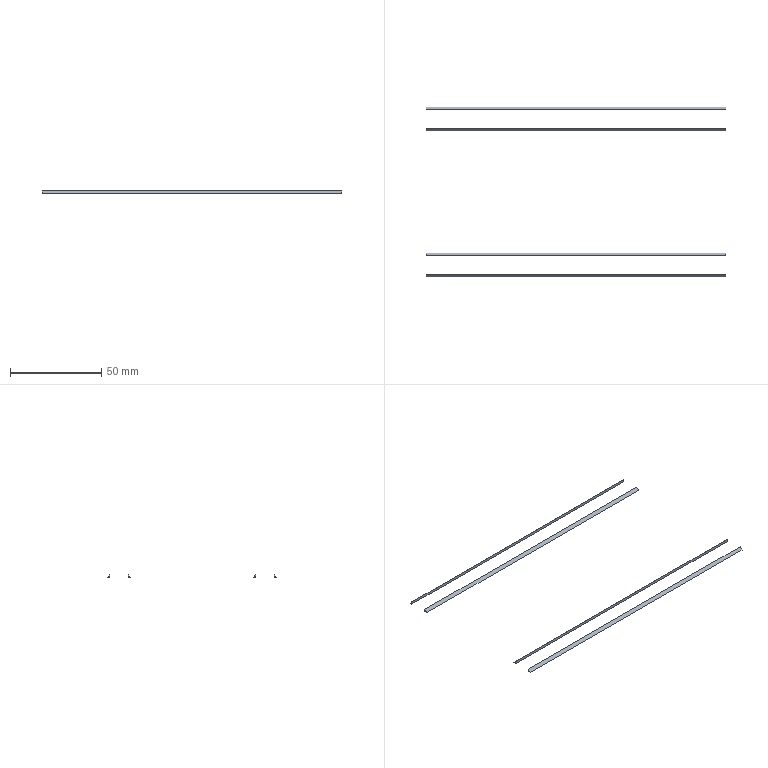Part | SolidWorks | features BaseBody 4 | 4 solids | 20 faces | box 164 x 93 x 1.5 mm | volume 738 mm3 | plane 20
STEP:
#1=CARTESIAN_POINT('',(152.,3.,6.4));
#2=VERTEX_POINT('',#1);
#3=CARTESIAN_POINT('',(152.,4.5,7.9));
#4=VERTEX_POINT('',#3);
#5=CARTESIAN_POINT('',(152.,4.5,7.9));
#6=DIRECTION('',(0.,0.7071,0.7071));
#7=VECTOR('',#6,1000.);
#8=LINE('',#5,#7);
#9=EDGE_CURVE('',#2,#4,#8,.T.);
#10=ORIENTED_EDGE('',*,*,#9,.T.);
#11=CARTESIAN_POINT('',(-12.,4.5,7.9));
#12=VERTEX_POINT('',#11);
#13=CARTESIAN_POINT('',(152.,4.5,7.9));
#14=DIRECTION('',(-1.,0.,0.));
#15=VECTOR('',#14,1000.);
#16=LINE('',#13,#15);
#17=EDGE_CURVE('',#4,#12,#16,.T.);
#18=ORIENTED_EDGE('',*,*,#17,.T.);
#19=CARTESIAN_POINT('',(-12.,3.,6.4));
#20=VERTEX_POINT('',#19);
#21=CARTESIAN_POINT('',(-12.,4.5,7.9));
#22=DIRECTION('',(0.,-0.7071,-0.7071));
#23=VECTOR('',#22,1000.);
#24=LINE('',#21,#23);
#25=EDGE_CURVE('',#12,#20,#24,.T.);
#26=ORIENTED_EDGE('',*,*,#25,.T.);
#27=CARTESIAN_POINT('',(152.,3.,6.4));
#28=DIRECTION('',(1.,0.,0.));
#29=VECTOR('',#28,1000.);
#30=LINE('',#27,#29);
#31=EDGE_CURVE('',#20,#2,#30,.T.);
#32=ORIENTED_EDGE('',*,*,#31,.T.);
#33=EDGE_LOOP('',(#10,#18,#26,#32));
#34=FACE_OUTER_BOUND('',#33,.T.);
#35=CARTESIAN_POINT('',(152.,4.5,7.9));
#36=DIRECTION('',(0.,-0.7071,0.7071));
#37=DIRECTION('',(0.,-0.7071,-0.7071));
#38=AXIS2_PLACEMENT_3D('',#35,#36,#37);
#39=PLANE('',#38);
#40=ADVANCED_FACE('',(#34),#39,.T.);
#41=CARTESIAN_POINT('',(152.,4.5,6.4));
#42=VERTEX_POINT('',#41);
#43=CARTESIAN_POINT('',(152.,4.5,6.4));
#44=DIRECTION('',(0.,0.,-1.));
#45=VECTOR('',#44,1000.);
#46=LINE('',#43,#45);
#47=EDGE_CURVE('',#4,#42,#46,.T.);
#48=ORIENTED_EDGE('',*,*,#47,.T.);
#49=CARTESIAN_POINT('',(-12.,4.5,6.4));
#50=VERTEX_POINT('',#49);
#51=CARTESIAN_POINT('',(152.,4.5,6.4));
#52=DIRECTION('',(-1.,0.,0.));
#53=VECTOR('',#52,1000.);
#54=LINE('',#51,#53);
#55=EDGE_CURVE('',#42,#50,#54,.T.);
#56=ORIENTED_EDGE('',*,*,#55,.T.);
#57=CARTESIAN_POINT('',(-12.,4.5,6.4));
#58=DIRECTION('',(0.,0.,1.));
#59=VECTOR('',#58,1000.);
#60=LINE('',#57,#59);
#61=EDGE_CURVE('',#50,#12,#60,.T.);
#62=ORIENTED_EDGE('',*,*,#61,.T.);
#63=ORIENTED_EDGE('',*,*,#17,.F.);
#64=EDGE_LOOP('',(#48,#56,#62,#63));
#65=FACE_OUTER_BOUND('',#64,.T.);
#66=CARTESIAN_POINT('',(152.,4.5,6.4));
#67=DIRECTION('',(0.,1.,0.));
#68=DIRECTION('',(-1.,0.,0.));
#69=AXIS2_PLACEMENT_3D('',#66,#67,#68);
#70=PLANE('',#69);
#71=ADVANCED_FACE('',(#65),#70,.T.);
#72=ORIENTED_EDGE('',*,*,#9,.F.);
#73=CARTESIAN_POINT('',(152.,3.97,6.4));
#74=DIRECTION('',(0.,1.,0.));
#75=VECTOR('',#74,1000.);
#76=LINE('',#73,#75);
#77=EDGE_CURVE('',#2,#42,#76,.T.);
#78=ORIENTED_EDGE('',*,*,#77,.T.);
#79=ORIENTED_EDGE('',*,*,#47,.F.);
#80=EDGE_LOOP('',(#72,#78,#79));
#81=FACE_OUTER_BOUND('',#80,.T.);
#82=CARTESIAN_POINT('',(152.,3.97,6.93));
#83=DIRECTION('',(1.,0.,0.));
#84=DIRECTION('',(0.,0.,-1.));
#85=AXIS2_PLACEMENT_3D('',#82,#83,#84);
#86=PLANE('',#85);
#87=ADVANCED_FACE('',(#81),#86,.T.);
#88=ORIENTED_EDGE('',*,*,#77,.F.);
#89=ORIENTED_EDGE('',*,*,#31,.F.);
#90=CARTESIAN_POINT('',(-12.,3.,6.4));
#91=DIRECTION('',(0.,1.,0.));
#92=VECTOR('',#91,1000.);
#93=LINE('',#90,#92);
#94=EDGE_CURVE('',#20,#50,#93,.T.);
#95=ORIENTED_EDGE('',*,*,#94,.T.);
#96=ORIENTED_EDGE('',*,*,#55,.F.);
#97=EDGE_LOOP('',(#88,#89,#95,#96));
#98=FACE_OUTER_BOUND('',#97,.T.);
#99=CARTESIAN_POINT('',(152.,3.,6.4));
#100=DIRECTION('',(0.,0.,-1.));
#101=DIRECTION('',(0.,1.,0.));
#102=AXIS2_PLACEMENT_3D('',#99,#100,#101);
#103=PLANE('',#102);
#104=ADVANCED_FACE('',(#98),#103,.T.);
#105=ORIENTED_EDGE('',*,*,#61,.F.);
#106=ORIENTED_EDGE('',*,*,#94,.F.);
#107=ORIENTED_EDGE('',*,*,#25,.F.);
#108=EDGE_LOOP('',(#105,#106,#107));
#109=FACE_OUTER_BOUND('',#108,.T.);
#110=CARTESIAN_POINT('',(-12.,3.97,6.93));
#111=DIRECTION('',(1.,0.,0.));
#112=DIRECTION('',(0.,0.,-1.));
#113=AXIS2_PLACEMENT_3D('',#110,#111,#112);
#114=PLANE('',#113);
#115=ADVANCED_FACE('',(#109),#114,.F.);
#116=CLOSED_SHELL('',(#40,#71,#87,#104,#115));
#117=MANIFOLD_SOLID_BREP('',#116);
#118=CARTESIAN_POINT('',(-12.,96.,6.4));
#119=VERTEX_POINT('',#118);
#120=CARTESIAN_POINT('',(-12.,94.5,7.9));
#121=VERTEX_POINT('',#120);
#122=CARTESIAN_POINT('',(-12.,94.5,7.9));
#123=DIRECTION('',(0.,-0.7071,0.7071));
#124=VECTOR('',#123,1000.);
#125=LINE('',#122,#124);
#126=EDGE_CURVE('',#119,#121,#125,.T.);
#127=ORIENTED_EDGE('',*,*,#126,.T.);
#128=CARTESIAN_POINT('',(152.,94.5,7.9));
#129=VERTEX_POINT('',#128);
#130=CARTESIAN_POINT('',(-12.,94.5,7.9));
#131=DIRECTION('',(1.,0.,0.));
#132=VECTOR('',#131,1000.);
#133=LINE('',#130,#132);
#134=EDGE_CURVE('',#121,#129,#133,.T.);
#135=ORIENTED_EDGE('',*,*,#134,.T.);
#136=CARTESIAN_POINT('',(152.,96.,6.4));
#137=VERTEX_POINT('',#136);
#138=CARTESIAN_POINT('',(152.,94.5,7.9));
#139=DIRECTION('',(0.,0.7071,-0.7071));
#140=VECTOR('',#139,1000.);
#141=LINE('',#138,#140);
#142=EDGE_CURVE('',#129,#137,#141,.T.);
#143=ORIENTED_EDGE('',*,*,#142,.T.);
#144=CARTESIAN_POINT('',(-12.,96.,6.4));
#145=DIRECTION('',(-1.,0.,0.));
#146=VECTOR('',#145,1000.);
#147=LINE('',#144,#146);
#148=EDGE_CURVE('',#137,#119,#147,.T.);
#149=ORIENTED_EDGE('',*,*,#148,.T.);
#150=EDGE_LOOP('',(#127,#135,#143,#149));
#151=FACE_OUTER_BOUND('',#150,.T.);
#152=CARTESIAN_POINT('',(-12.,94.5,7.9));
#153=DIRECTION('',(0.,0.7071,0.7071));
#154=DIRECTION('',(0.,-0.7071,0.7071));
#155=AXIS2_PLACEMENT_3D('',#152,#153,#154);
#156=PLANE('',#155);
#157=ADVANCED_FACE('',(#151),#156,.T.);
#158=CARTESIAN_POINT('',(-12.,94.5,6.4));
#159=VERTEX_POINT('',#158);
#160=CARTESIAN_POINT('',(-12.,94.5,6.4));
#161=DIRECTION('',(0.,0.,-1.));
#162=VECTOR('',#161,1000.);
#163=LINE('',#160,#162);
#164=EDGE_CURVE('',#121,#159,#163,.T.);
#165=ORIENTED_EDGE('',*,*,#164,.T.);
#166=CARTESIAN_POINT('',(152.,94.5,6.4));
#167=VERTEX_POINT('',#166);
#168=CARTESIAN_POINT('',(-12.,94.5,6.4));
#169=DIRECTION('',(1.,0.,0.));
#170=VECTOR('',#169,1000.);
#171=LINE('',#168,#170);
#172=EDGE_CURVE('',#159,#167,#171,.T.);
#173=ORIENTED_EDGE('',*,*,#172,.T.);
#174=CARTESIAN_POINT('',(152.,94.5,6.4));
#175=DIRECTION('',(0.,0.,1.));
#176=VECTOR('',#175,1000.);
#177=LINE('',#174,#176);
#178=EDGE_CURVE('',#167,#129,#177,.T.);
#179=ORIENTED_EDGE('',*,*,#178,.T.);
#180=ORIENTED_EDGE('',*,*,#134,.F.);
#181=EDGE_LOOP('',(#165,#173,#179,#180));
#182=FACE_OUTER_BOUND('',#181,.T.);
#183=CARTESIAN_POINT('',(-12.,94.5,6.4));
#184=DIRECTION('',(0.,-1.,0.));
#185=DIRECTION('',(1.,0.,0.));
#186=AXIS2_PLACEMENT_3D('',#183,#184,#185);
#187=PLANE('',#186);
#188=ADVANCED_FACE('',(#182),#187,.T.);
#189=ORIENTED_EDGE('',*,*,#126,.F.);
#190=CARTESIAN_POINT('',(-12.,95.03,6.4));
#191=DIRECTION('',(0.,1.,0.));
#192=VECTOR('',#191,1000.);
#193=LINE('',#190,#192);
#194=EDGE_CURVE('',#159,#119,#193,.T.);
#195=ORIENTED_EDGE('',*,*,#194,.F.);
#196=ORIENTED_EDGE('',*,*,#164,.F.);
#197=EDGE_LOOP('',(#189,#195,#196));
#198=FACE_OUTER_BOUND('',#197,.T.);
#199=CARTESIAN_POINT('',(-12.,95.03,6.93));
#200=DIRECTION('',(1.,0.,0.));
#201=DIRECTION('',(0.,0.,-1.));
#202=AXIS2_PLACEMENT_3D('',#199,#200,#201);
#203=PLANE('',#202);
#204=ADVANCED_FACE('',(#198),#203,.F.);
#205=ORIENTED_EDGE('',*,*,#194,.T.);
#206=ORIENTED_EDGE('',*,*,#148,.F.);
#207=CARTESIAN_POINT('',(152.,96.,6.4));
#208=DIRECTION('',(0.,-1.,0.));
#209=VECTOR('',#208,1000.);
#210=LINE('',#207,#209);
#211=EDGE_CURVE('',#137,#167,#210,.T.);
#212=ORIENTED_EDGE('',*,*,#211,.T.);
#213=ORIENTED_EDGE('',*,*,#172,.F.);
#214=EDGE_LOOP('',(#205,#206,#212,#213));
#215=FACE_OUTER_BOUND('',#214,.T.);
#216=CARTESIAN_POINT('',(-12.,96.,6.4));
#217=DIRECTION('',(0.,0.,-1.));
#218=DIRECTION('',(0.,1.,0.));
#219=AXIS2_PLACEMENT_3D('',#216,#217,#218);
#220=PLANE('',#219);
#221=ADVANCED_FACE('',(#215),#220,.T.);
#222=ORIENTED_EDGE('',*,*,#178,.F.);
#223=ORIENTED_EDGE('',*,*,#211,.F.);
#224=ORIENTED_EDGE('',*,*,#142,.F.);
#225=EDGE_LOOP('',(#222,#223,#224));
#226=FACE_OUTER_BOUND('',#225,.T.);
#227=CARTESIAN_POINT('',(152.,95.03,6.93));
#228=DIRECTION('',(1.,0.,0.));
#229=DIRECTION('',(0.,0.,-1.));
#230=AXIS2_PLACEMENT_3D('',#227,#228,#229);
#231=PLANE('',#230);
#232=ADVANCED_FACE('',(#226),#231,.T.);
#233=CLOSED_SHELL('',(#157,#188,#204,#221,#232));
#234=MANIFOLD_SOLID_BREP('',#233);
#235=CARTESIAN_POINT('',(-12.,16.,6.4));
#236=VERTEX_POINT('',#235);
#237=CARTESIAN_POINT('',(-12.,14.5,7.9));
#238=VERTEX_POINT('',#237);
#239=CARTESIAN_POINT('',(-12.,14.5,7.9));
#240=DIRECTION('',(0.,-0.7071,0.7071));
#241=VECTOR('',#240,1000.);
#242=LINE('',#239,#241);
#243=EDGE_CURVE('',#236,#238,#242,.T.);
#244=ORIENTED_EDGE('',*,*,#243,.T.);
#245=CARTESIAN_POINT('',(152.,14.5,7.9));
#246=VERTEX_POINT('',#245);
#247=CARTESIAN_POINT('',(-12.,14.5,7.9));
#248=DIRECTION('',(1.,0.,0.));
#249=VECTOR('',#248,1000.);
#250=LINE('',#247,#249);
#251=EDGE_CURVE('',#238,#246,#250,.T.);
#252=ORIENTED_EDGE('',*,*,#251,.T.);
#253=CARTESIAN_POINT('',(152.,16.,6.4));
#254=VERTEX_POINT('',#253);
#255=CARTESIAN_POINT('',(152.,14.5,7.9));
#256=DIRECTION('',(0.,0.7071,-0.7071));
#257=VECTOR('',#256,1000.);
#258=LINE('',#255,#257);
#259=EDGE_CURVE('',#246,#254,#258,.T.);
#260=ORIENTED_EDGE('',*,*,#259,.T.);
#261=CARTESIAN_POINT('',(-12.,16.,6.4));
#262=DIRECTION('',(-1.,0.,0.));
#263=VECTOR('',#262,1000.);
#264=LINE('',#261,#263);
#265=EDGE_CURVE('',#254,#236,#264,.T.);
#266=ORIENTED_EDGE('',*,*,#265,.T.);
#267=EDGE_LOOP('',(#244,#252,#260,#266));
#268=FACE_OUTER_BOUND('',#267,.T.);
#269=CARTESIAN_POINT('',(-12.,14.5,7.9));
#270=DIRECTION('',(0.,0.7071,0.7071));
#271=DIRECTION('',(0.,-0.7071,0.7071));
#272=AXIS2_PLACEMENT_3D('',#269,#270,#271);
#273=PLANE('',#272);
#274=ADVANCED_FACE('',(#268),#273,.T.);
#275=CARTESIAN_POINT('',(-12.,14.5,6.4));
#276=VERTEX_POINT('',#275);
#277=CARTESIAN_POINT('',(-12.,14.5,6.4));
#278=DIRECTION('',(0.,0.,-1.));
#279=VECTOR('',#278,1000.);
#280=LINE('',#277,#279);
#281=EDGE_CURVE('',#238,#276,#280,.T.);
#282=ORIENTED_EDGE('',*,*,#281,.T.);
#283=CARTESIAN_POINT('',(152.,14.5,6.4));
#284=VERTEX_POINT('',#283);
#285=CARTESIAN_POINT('',(-12.,14.5,6.4));
#286=DIRECTION('',(1.,0.,0.));
#287=VECTOR('',#286,1000.);
#288=LINE('',#285,#287);
#289=EDGE_CURVE('',#276,#284,#288,.T.);
#290=ORIENTED_EDGE('',*,*,#289,.T.);
#291=CARTESIAN_POINT('',(152.,14.5,6.4));
#292=DIRECTION('',(0.,0.,1.));
#293=VECTOR('',#292,1000.);
#294=LINE('',#291,#293);
#295=EDGE_CURVE('',#284,#246,#294,.T.);
#296=ORIENTED_EDGE('',*,*,#295,.T.);
#297=ORIENTED_EDGE('',*,*,#251,.F.);
#298=EDGE_LOOP('',(#282,#290,#296,#297));
#299=FACE_OUTER_BOUND('',#298,.T.);
#300=CARTESIAN_POINT('',(-12.,14.5,6.4));
#301=DIRECTION('',(0.,-1.,0.));
#302=DIRECTION('',(1.,0.,0.));
#303=AXIS2_PLACEMENT_3D('',#300,#301,#302);
#304=PLANE('',#303);
#305=ADVANCED_FACE('',(#299),#304,.T.);
#306=ORIENTED_EDGE('',*,*,#243,.F.);
#307=CARTESIAN_POINT('',(-12.,15.03,6.4));
#308=DIRECTION('',(0.,1.,0.));
#309=VECTOR('',#308,1000.);
#310=LINE('',#307,#309);
#311=EDGE_CURVE('',#276,#236,#310,.T.);
#312=ORIENTED_EDGE('',*,*,#311,.F.);
#313=ORIENTED_EDGE('',*,*,#281,.F.);
#314=EDGE_LOOP('',(#306,#312,#313));
#315=FACE_OUTER_BOUND('',#314,.T.);
#316=CARTESIAN_POINT('',(-12.,15.03,6.93));
#317=DIRECTION('',(1.,0.,0.));
#318=DIRECTION('',(0.,0.,-1.));
#319=AXIS2_PLACEMENT_3D('',#316,#317,#318);
#320=PLANE('',#319);
#321=ADVANCED_FACE('',(#315),#320,.F.);
#322=ORIENTED_EDGE('',*,*,#311,.T.);
#323=ORIENTED_EDGE('',*,*,#265,.F.);
#324=CARTESIAN_POINT('',(152.,16.,6.4));
#325=DIRECTION('',(0.,-1.,0.));
#326=VECTOR('',#325,1000.);
#327=LINE('',#324,#326);
#328=EDGE_CURVE('',#254,#284,#327,.T.);
#329=ORIENTED_EDGE('',*,*,#328,.T.);
#330=ORIENTED_EDGE('',*,*,#289,.F.);
#331=EDGE_LOOP('',(#322,#323,#329,#330));
#332=FACE_OUTER_BOUND('',#331,.T.);
#333=CARTESIAN_POINT('',(-12.,16.,6.4));
#334=DIRECTION('',(0.,0.,-1.));
#335=DIRECTION('',(0.,1.,0.));
#336=AXIS2_PLACEMENT_3D('',#333,#334,#335);
#337=PLANE('',#336);
#338=ADVANCED_FACE('',(#332),#337,.T.);
#339=ORIENTED_EDGE('',*,*,#295,.F.);
#340=ORIENTED_EDGE('',*,*,#328,.F.);
#341=ORIENTED_EDGE('',*,*,#259,.F.);
#342=EDGE_LOOP('',(#339,#340,#341));
#343=FACE_OUTER_BOUND('',#342,.T.);
#344=CARTESIAN_POINT('',(152.,15.03,6.93));
#345=DIRECTION('',(1.,0.,0.));
#346=DIRECTION('',(0.,0.,-1.));
#347=AXIS2_PLACEMENT_3D('',#344,#345,#346);
#348=PLANE('',#347);
#349=ADVANCED_FACE('',(#343),#348,.T.);
#350=CLOSED_SHELL('',(#274,#305,#321,#338,#349));
#351=MANIFOLD_SOLID_BREP('',#350);
#352=CARTESIAN_POINT('',(152.,83.,6.4));
#353=VERTEX_POINT('',#352);
#354=CARTESIAN_POINT('',(152.,84.5,7.9));
#355=VERTEX_POINT('',#354);
#356=CARTESIAN_POINT('',(152.,84.5,7.9));
#357=DIRECTION('',(0.,0.7071,0.7071));
#358=VECTOR('',#357,1000.);
#359=LINE('',#356,#358);
#360=EDGE_CURVE('',#353,#355,#359,.T.);
#361=ORIENTED_EDGE('',*,*,#360,.T.);
#362=CARTESIAN_POINT('',(-12.,84.5,7.9));
#363=VERTEX_POINT('',#362);
#364=CARTESIAN_POINT('',(152.,84.5,7.9));
#365=DIRECTION('',(-1.,0.,0.));
#366=VECTOR('',#365,1000.);
#367=LINE('',#364,#366);
#368=EDGE_CURVE('',#355,#363,#367,.T.);
#369=ORIENTED_EDGE('',*,*,#368,.T.);
#370=CARTESIAN_POINT('',(-12.,83.,6.4));
#371=VERTEX_POINT('',#370);
#372=CARTESIAN_POINT('',(-12.,84.5,7.9));
#373=DIRECTION('',(0.,-0.7071,-0.7071));
#374=VECTOR('',#373,1000.);
#375=LINE('',#372,#374);
#376=EDGE_CURVE('',#363,#371,#375,.T.);
#377=ORIENTED_EDGE('',*,*,#376,.T.);
#378=CARTESIAN_POINT('',(152.,83.,6.4));
#379=DIRECTION('',(1.,0.,0.));
#380=VECTOR('',#379,1000.);
#381=LINE('',#378,#380);
#382=EDGE_CURVE('',#371,#353,#381,.T.);
#383=ORIENTED_EDGE('',*,*,#382,.T.);
#384=EDGE_LOOP('',(#361,#369,#377,#383));
#385=FACE_OUTER_BOUND('',#384,.T.);
#386=CARTESIAN_POINT('',(152.,84.5,7.9));
#387=DIRECTION('',(0.,-0.7071,0.7071));
#388=DIRECTION('',(0.,-0.7071,-0.7071));
#389=AXIS2_PLACEMENT_3D('',#386,#387,#388);
#390=PLANE('',#389);
#391=ADVANCED_FACE('',(#385),#390,.T.);
#392=CARTESIAN_POINT('',(152.,84.5,6.4));
#393=VERTEX_POINT('',#392);
#394=CARTESIAN_POINT('',(152.,84.5,6.4));
#395=DIRECTION('',(0.,0.,-1.));
#396=VECTOR('',#395,1000.);
#397=LINE('',#394,#396);
#398=EDGE_CURVE('',#355,#393,#397,.T.);
#399=ORIENTED_EDGE('',*,*,#398,.T.);
#400=CARTESIAN_POINT('',(-12.,84.5,6.4));
#401=VERTEX_POINT('',#400);
#402=CARTESIAN_POINT('',(152.,84.5,6.4));
#403=DIRECTION('',(-1.,0.,0.));
#404=VECTOR('',#403,1000.);
#405=LINE('',#402,#404);
#406=EDGE_CURVE('',#393,#401,#405,.T.);
#407=ORIENTED_EDGE('',*,*,#406,.T.);
#408=CARTESIAN_POINT('',(-12.,84.5,6.4));
#409=DIRECTION('',(0.,0.,1.));
#410=VECTOR('',#409,1000.);
#411=LINE('',#408,#410);
#412=EDGE_CURVE('',#401,#363,#411,.T.);
#413=ORIENTED_EDGE('',*,*,#412,.T.);
#414=ORIENTED_EDGE('',*,*,#368,.F.);
#415=EDGE_LOOP('',(#399,#407,#413,#414));
#416=FACE_OUTER_BOUND('',#415,.T.);
#417=CARTESIAN_POINT('',(152.,84.5,6.4));
#418=DIRECTION('',(0.,1.,0.));
#419=DIRECTION('',(-1.,0.,0.));
#420=AXIS2_PLACEMENT_3D('',#417,#418,#419);
#421=PLANE('',#420);
#422=ADVANCED_FACE('',(#416),#421,.T.);
#423=ORIENTED_EDGE('',*,*,#360,.F.);
#424=CARTESIAN_POINT('',(152.,83.97,6.4));
#425=DIRECTION('',(0.,1.,0.));
#426=VECTOR('',#425,1000.);
#427=LINE('',#424,#426);
#428=EDGE_CURVE('',#353,#393,#427,.T.);
#429=ORIENTED_EDGE('',*,*,#428,.T.);
#430=ORIENTED_EDGE('',*,*,#398,.F.);
#431=EDGE_LOOP('',(#423,#429,#430));
#432=FACE_OUTER_BOUND('',#431,.T.);
#433=CARTESIAN_POINT('',(152.,83.97,6.93));
#434=DIRECTION('',(1.,0.,0.));
#435=DIRECTION('',(0.,0.,-1.));
#436=AXIS2_PLACEMENT_3D('',#433,#434,#435);
#437=PLANE('',#436);
#438=ADVANCED_FACE('',(#432),#437,.T.);
#439=ORIENTED_EDGE('',*,*,#428,.F.);
#440=ORIENTED_EDGE('',*,*,#382,.F.);
#441=CARTESIAN_POINT('',(-12.,83.,6.4));
#442=DIRECTION('',(0.,1.,0.));
#443=VECTOR('',#442,1000.);
#444=LINE('',#441,#443);
#445=EDGE_CURVE('',#371,#401,#444,.T.);
#446=ORIENTED_EDGE('',*,*,#445,.T.);
#447=ORIENTED_EDGE('',*,*,#406,.F.);
#448=EDGE_LOOP('',(#439,#440,#446,#447));
#449=FACE_OUTER_BOUND('',#448,.T.);
#450=CARTESIAN_POINT('',(152.,83.,6.4));
#451=DIRECTION('',(0.,0.,-1.));
#452=DIRECTION('',(0.,1.,0.));
#453=AXIS2_PLACEMENT_3D('',#450,#451,#452);
#454=PLANE('',#453);
#455=ADVANCED_FACE('',(#449),#454,.T.);
#456=ORIENTED_EDGE('',*,*,#412,.F.);
#457=ORIENTED_EDGE('',*,*,#445,.F.);
#458=ORIENTED_EDGE('',*,*,#376,.F.);
#459=EDGE_LOOP('',(#456,#457,#458));
#460=FACE_OUTER_BOUND('',#459,.T.);
#461=CARTESIAN_POINT('',(-12.,83.97,6.93));
#462=DIRECTION('',(1.,0.,0.));
#463=DIRECTION('',(0.,0.,-1.));
#464=AXIS2_PLACEMENT_3D('',#461,#462,#463);
#465=PLANE('',#464);
#466=ADVANCED_FACE('',(#460),#465,.F.);
#467=CLOSED_SHELL('',(#391,#422,#438,#455,#466));
#468=MANIFOLD_SOLID_BREP('',#467);
#469=CARTESIAN_POINT('',(0.,0.,0.));
#470=DIRECTION('',(0.,0.,1.));
#471=DIRECTION('',(1.,0.,0.));
#472=AXIS2_PLACEMENT_3D('',#469,#470,#471);
#473=(LENGTH_UNIT()NAMED_UNIT(*)SI_UNIT(.MILLI.,.METRE.));
#474=UNCERTAINTY_MEASURE_WITH_UNIT(LENGTH_MEASURE(0.00001),#473,'','');
#475=(NAMED_UNIT(*)PLANE_ANGLE_UNIT()SI_UNIT($,.RADIAN.));
#476=(NAMED_UNIT(*)SI_UNIT($,.STERADIAN.)SOLID_ANGLE_UNIT());
#477=(GEOMETRIC_REPRESENTATION_CONTEXT(3)GLOBAL_UNCERTAINTY_ASSIGNED_CONTEXT((#474))GLOBAL_UNIT_ASSIGNED_CONTEXT((#473,#475,#476))REPRESENTATION_CONTEXT('',''));
#478=ADVANCED_BREP_SHAPE_REPRESENTATION('',(#117,#234,#351,#468,#472),#477);